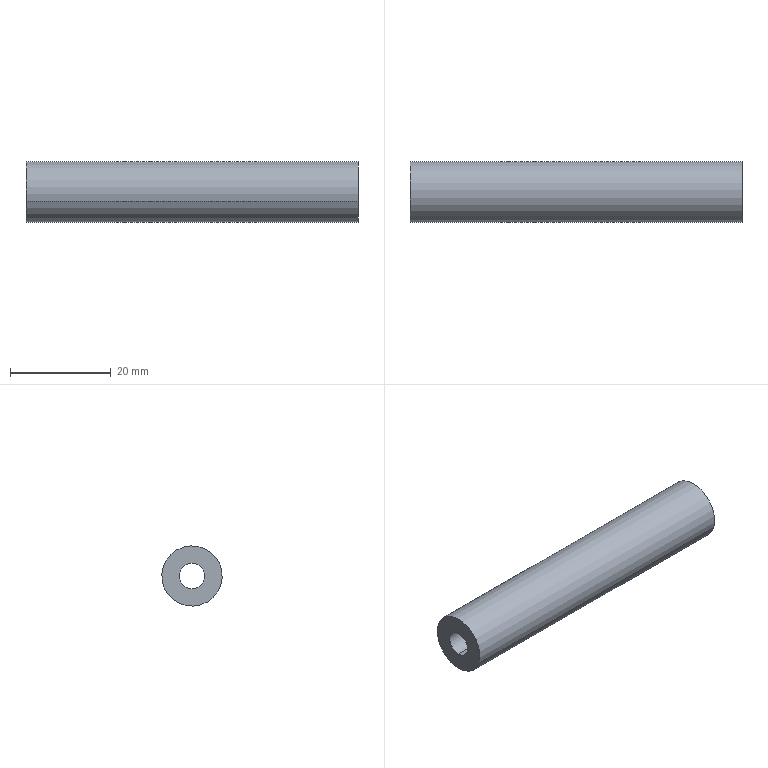Part | STEP file | Previa 01.sldasm-Part-10_Valor predeterminado | 1 solid | 6 faces | box 66 x 12 x 12 mm | volume 6169 mm3 | cylinder 4 | plane 2 | commonest cylinder face diameters 5 x2 12 x2
STEP:
#1=CARTESIAN_POINT('',(0.,0.,0.));
#2=DIRECTION('',(0.,0.,1.));
#3=DIRECTION('',(1.,0.,0.));
#4=AXIS2_PLACEMENT_3D('',#1,#2,#3);
#5=CARTESIAN_POINT('',(-100.103,41.846,11.097));
#6=VERTEX_POINT('',#5);
#7=CARTESIAN_POINT('',(-34.103,41.846,11.097));
#8=VERTEX_POINT('',#7);
#9=CARTESIAN_POINT('',(-34.103,41.846,11.097));
#10=DIRECTION('',(1.,0.,0.));
#11=VECTOR('',#10,1.);
#12=LINE('',#9,#11);
#13=CARTESIAN_POINT('',(-34.103,41.846,13.597));
#14=DIRECTION('',(1.,0.,0.));
#15=DIRECTION('',(0.,0.,-1.));
#16=AXIS2_PLACEMENT_3D('',#13,#14,#15);
#17=CYLINDRICAL_SURFACE('',#16,2.5);
#18=CARTESIAN_POINT('',(6.283,0.));
#19=DIRECTION('',(0.,1.));
#20=VECTOR('',#19,1.);
#21=LINE('',#18,#20);
#22=(GEOMETRIC_REPRESENTATION_CONTEXT(2)PARAMETRIC_REPRESENTATION_CONTEXT()REPRESENTATION_CONTEXT('',''));
#23=DEFINITIONAL_REPRESENTATION('',(#21),#22);
#24=PCURVE('',#17,#23);
#25=CARTESIAN_POINT('',(-34.103,41.846,13.597));
#26=DIRECTION('',(1.,0.,0.));
#27=DIRECTION('',(0.,0.,-1.));
#28=AXIS2_PLACEMENT_3D('',#25,#26,#27);
#29=CYLINDRICAL_SURFACE('',#28,2.5);
#30=CARTESIAN_POINT('',(0.,0.));
#31=DIRECTION('',(0.,1.));
#32=VECTOR('',#31,1.);
#33=LINE('',#30,#32);
#34=(GEOMETRIC_REPRESENTATION_CONTEXT(2)PARAMETRIC_REPRESENTATION_CONTEXT()REPRESENTATION_CONTEXT('',''));
#35=DEFINITIONAL_REPRESENTATION('',(#33),#34);
#36=PCURVE('',#29,#35);
#37=SURFACE_CURVE('',#12,(#24,#36),.PCURVE_S1.);
#38=EDGE_CURVE('',#6,#8,#37,.T.);
#39=ORIENTED_EDGE('',*,*,#38,.T.);
#40=CARTESIAN_POINT('',(-34.103,41.846,16.097));
#41=VERTEX_POINT('',#40);
#42=CARTESIAN_POINT('',(-34.103,41.846,13.597));
#43=DIRECTION('',(1.,0.,0.));
#44=DIRECTION('',(0.,0.,-1.));
#45=AXIS2_PLACEMENT_3D('',#42,#43,#44);
#46=CIRCLE('',#45,2.5);
#47=CARTESIAN_POINT('',(0.,0.));
#48=DIRECTION('',(1.,0.));
#49=VECTOR('',#48,1.);
#50=LINE('',#47,#49);
#51=(GEOMETRIC_REPRESENTATION_CONTEXT(2)PARAMETRIC_REPRESENTATION_CONTEXT()REPRESENTATION_CONTEXT('',''));
#52=DEFINITIONAL_REPRESENTATION('',(#50),#51);
#53=PCURVE('',#17,#52);
#54=CARTESIAN_POINT('',(-34.103,41.846,13.597));
#55=DIRECTION('',(-1.,0.,0.));
#56=DIRECTION('',(0.,0.9511,0.309));
#57=AXIS2_PLACEMENT_3D('',#54,#55,#56);
#58=PLANE('',#57);
#59=CARTESIAN_POINT('',(-0.7725,2.378));
#60=CARTESIAN_POINT('',(3.346,3.716));
#61=CARTESIAN_POINT('',(2.445,-0.5198));
#62=CARTESIAN_POINT('',(1.545,-4.755));
#63=CARTESIAN_POINT('',(-1.673,-1.858));
#64=CARTESIAN_POINT('',(-4.891,1.04));
#65=CARTESIAN_POINT('',(-0.7725,2.378));
#66=(BOUNDED_CURVE()B_SPLINE_CURVE(2,(#59,#60,#61,#62,#63,#64,#65),.UNSPECIFIED.,.T.,.F.)B_SPLINE_CURVE_WITH_KNOTS((1,2,2,2,2,1),(-2.094,0.,2.094,4.189,6.283,8.378),.UNSPECIFIED.)CURVE()GEOMETRIC_REPRESENTATION_ITEM()RATIONAL_B_SPLINE_CURVE((1.,0.5,1.,0.5,1.,0.5,1.))REPRESENTATION_ITEM(''));
#67=(GEOMETRIC_REPRESENTATION_CONTEXT(2)PARAMETRIC_REPRESENTATION_CONTEXT()REPRESENTATION_CONTEXT('',''));
#68=DEFINITIONAL_REPRESENTATION('',(#66),#67);
#69=PCURVE('',#58,#68);
#70=SURFACE_CURVE('',#46,(#53,#69),.PCURVE_S1.);
#71=EDGE_CURVE('',#41,#8,#70,.T.);
#72=ORIENTED_EDGE('',*,*,#71,.F.);
#73=CARTESIAN_POINT('',(-100.103,41.846,16.097));
#74=VERTEX_POINT('',#73);
#75=CARTESIAN_POINT('',(-34.103,41.846,16.097));
#76=DIRECTION('',(1.,0.,0.));
#77=VECTOR('',#76,1.);
#78=LINE('',#75,#77);
#79=CARTESIAN_POINT('',(3.142,0.));
#80=DIRECTION('',(0.,1.));
#81=VECTOR('',#80,1.);
#82=LINE('',#79,#81);
#83=(GEOMETRIC_REPRESENTATION_CONTEXT(2)PARAMETRIC_REPRESENTATION_CONTEXT()REPRESENTATION_CONTEXT('',''));
#84=DEFINITIONAL_REPRESENTATION('',(#82),#83);
#85=PCURVE('',#17,#84);
#86=CARTESIAN_POINT('',(3.142,0.));
#87=DIRECTION('',(0.,1.));
#88=VECTOR('',#87,1.);
#89=LINE('',#86,#88);
#90=(GEOMETRIC_REPRESENTATION_CONTEXT(2)PARAMETRIC_REPRESENTATION_CONTEXT()REPRESENTATION_CONTEXT('',''));
#91=DEFINITIONAL_REPRESENTATION('',(#89),#90);
#92=PCURVE('',#29,#91);
#93=SURFACE_CURVE('',#78,(#85,#92),.PCURVE_S1.);
#94=EDGE_CURVE('',#74,#41,#93,.T.);
#95=ORIENTED_EDGE('',*,*,#94,.F.);
#96=CARTESIAN_POINT('',(-100.103,41.846,13.597));
#97=DIRECTION('',(1.,0.,0.));
#98=DIRECTION('',(0.,0.,-1.));
#99=AXIS2_PLACEMENT_3D('',#96,#97,#98);
#100=CIRCLE('',#99,2.5);
#101=CARTESIAN_POINT('',(0.,-66.));
#102=DIRECTION('',(1.,0.));
#103=VECTOR('',#102,1.);
#104=LINE('',#101,#103);
#105=(GEOMETRIC_REPRESENTATION_CONTEXT(2)PARAMETRIC_REPRESENTATION_CONTEXT()REPRESENTATION_CONTEXT('',''));
#106=DEFINITIONAL_REPRESENTATION('',(#104),#105);
#107=PCURVE('',#17,#106);
#108=CARTESIAN_POINT('',(-100.103,41.846,13.597));
#109=DIRECTION('',(-1.,0.,0.));
#110=DIRECTION('',(0.,0.9511,0.309));
#111=AXIS2_PLACEMENT_3D('',#108,#109,#110);
#112=PLANE('',#111);
#113=CARTESIAN_POINT('',(-0.7725,2.378));
#114=CARTESIAN_POINT('',(3.346,3.716));
#115=CARTESIAN_POINT('',(2.445,-0.5198));
#116=CARTESIAN_POINT('',(1.545,-4.755));
#117=CARTESIAN_POINT('',(-1.673,-1.858));
#118=CARTESIAN_POINT('',(-4.891,1.04));
#119=CARTESIAN_POINT('',(-0.7725,2.378));
#120=(BOUNDED_CURVE()B_SPLINE_CURVE(2,(#113,#114,#115,#116,#117,#118,#119),.UNSPECIFIED.,.T.,.F.)B_SPLINE_CURVE_WITH_KNOTS((1,2,2,2,2,1),(-2.094,0.,2.094,4.189,6.283,8.378),.UNSPECIFIED.)CURVE()GEOMETRIC_REPRESENTATION_ITEM()RATIONAL_B_SPLINE_CURVE((1.,0.5,1.,0.5,1.,0.5,1.))REPRESENTATION_ITEM(''));
#121=(GEOMETRIC_REPRESENTATION_CONTEXT(2)PARAMETRIC_REPRESENTATION_CONTEXT()REPRESENTATION_CONTEXT('',''));
#122=DEFINITIONAL_REPRESENTATION('',(#120),#121);
#123=PCURVE('',#112,#122);
#124=SURFACE_CURVE('',#100,(#107,#123),.PCURVE_S1.);
#125=EDGE_CURVE('',#74,#6,#124,.T.);
#126=ORIENTED_EDGE('',*,*,#125,.T.);
#127=EDGE_LOOP('',(#39,#72,#95,#126));
#128=FACE_BOUND('',#127,.F.);
#129=ADVANCED_FACE('',(#128),#17,.F.);
#130=CARTESIAN_POINT('',(-100.103,47.553,15.451));
#131=VERTEX_POINT('',#130);
#132=CARTESIAN_POINT('',(-100.103,36.14,11.743));
#133=VERTEX_POINT('',#132);
#134=CARTESIAN_POINT('',(-100.103,41.846,13.597));
#135=DIRECTION('',(-1.,0.,0.));
#136=DIRECTION('',(0.,0.,1.));
#137=AXIS2_PLACEMENT_3D('',#134,#135,#136);
#138=CIRCLE('',#137,6.);
#139=CARTESIAN_POINT('',(-162.103,41.846,13.597));
#140=DIRECTION('',(1.,0.,0.));
#141=DIRECTION('',(0.,-0.9511,-0.309));
#142=AXIS2_PLACEMENT_3D('',#139,#140,#141);
#143=CYLINDRICAL_SURFACE('',#142,6.);
#144=CARTESIAN_POINT('',(4.398,62.));
#145=DIRECTION('',(-1.,0.));
#146=VECTOR('',#145,1.);
#147=LINE('',#144,#146);
#148=(GEOMETRIC_REPRESENTATION_CONTEXT(2)PARAMETRIC_REPRESENTATION_CONTEXT()REPRESENTATION_CONTEXT('',''));
#149=DEFINITIONAL_REPRESENTATION('',(#147),#148);
#150=PCURVE('',#143,#149);
#151=CARTESIAN_POINT('',(0.,0.));
#152=DIRECTION('',(0.309,-0.9511));
#153=AXIS2_PLACEMENT_2D('',#151,#152);
#154=CIRCLE('',#153,6.);
#155=(GEOMETRIC_REPRESENTATION_CONTEXT(2)PARAMETRIC_REPRESENTATION_CONTEXT()REPRESENTATION_CONTEXT('',''));
#156=DEFINITIONAL_REPRESENTATION('',(#154),#155);
#157=PCURVE('',#112,#156);
#158=SURFACE_CURVE('',#138,(#150,#157),.PCURVE_S1.);
#159=EDGE_CURVE('',#131,#133,#158,.T.);
#160=ORIENTED_EDGE('',*,*,#159,.F.);
#161=CARTESIAN_POINT('',(-34.103,47.553,15.451));
#162=VERTEX_POINT('',#161);
#163=CARTESIAN_POINT('',(-162.103,47.553,15.451));
#164=DIRECTION('',(1.,0.,0.));
#165=VECTOR('',#164,1.);
#166=LINE('',#163,#165);
#167=CARTESIAN_POINT('',(3.142,0.));
#168=DIRECTION('',(0.,1.));
#169=VECTOR('',#168,1.);
#170=LINE('',#167,#169);
#171=(GEOMETRIC_REPRESENTATION_CONTEXT(2)PARAMETRIC_REPRESENTATION_CONTEXT()REPRESENTATION_CONTEXT('',''));
#172=DEFINITIONAL_REPRESENTATION('',(#170),#171);
#173=PCURVE('',#143,#172);
#174=CARTESIAN_POINT('',(-162.103,41.846,13.597));
#175=DIRECTION('',(1.,0.,0.));
#176=DIRECTION('',(0.,-0.9511,-0.309));
#177=AXIS2_PLACEMENT_3D('',#174,#175,#176);
#178=CYLINDRICAL_SURFACE('',#177,6.);
#179=CARTESIAN_POINT('',(3.142,0.));
#180=DIRECTION('',(0.,1.));
#181=VECTOR('',#180,1.);
#182=LINE('',#179,#181);
#183=(GEOMETRIC_REPRESENTATION_CONTEXT(2)PARAMETRIC_REPRESENTATION_CONTEXT()REPRESENTATION_CONTEXT('',''));
#184=DEFINITIONAL_REPRESENTATION('',(#182),#183);
#185=PCURVE('',#178,#184);
#186=SURFACE_CURVE('',#166,(#173,#185),.PCURVE_S1.);
#187=EDGE_CURVE('',#131,#162,#186,.T.);
#188=ORIENTED_EDGE('',*,*,#187,.T.);
#189=CARTESIAN_POINT('',(-34.103,36.14,11.743));
#190=VERTEX_POINT('',#189);
#191=CARTESIAN_POINT('',(-34.103,41.846,13.597));
#192=DIRECTION('',(-1.,0.,0.));
#193=DIRECTION('',(0.,-0.309,0.9511));
#194=AXIS2_PLACEMENT_3D('',#191,#192,#193);
#195=CIRCLE('',#194,6.);
#196=CARTESIAN_POINT('',(4.712,128.));
#197=DIRECTION('',(-1.,0.));
#198=VECTOR('',#197,1.);
#199=LINE('',#196,#198);
#200=(GEOMETRIC_REPRESENTATION_CONTEXT(2)PARAMETRIC_REPRESENTATION_CONTEXT()REPRESENTATION_CONTEXT('',''));
#201=DEFINITIONAL_REPRESENTATION('',(#199),#200);
#202=PCURVE('',#143,#201);
#203=CARTESIAN_POINT('',(0.,0.));
#204=DIRECTION('',(0.,-1.));
#205=AXIS2_PLACEMENT_2D('',#203,#204);
#206=CIRCLE('',#205,6.);
#207=(GEOMETRIC_REPRESENTATION_CONTEXT(2)PARAMETRIC_REPRESENTATION_CONTEXT()REPRESENTATION_CONTEXT('',''));
#208=DEFINITIONAL_REPRESENTATION('',(#206),#207);
#209=PCURVE('',#58,#208);
#210=SURFACE_CURVE('',#195,(#202,#209),.PCURVE_S1.);
#211=EDGE_CURVE('',#162,#190,#210,.T.);
#212=ORIENTED_EDGE('',*,*,#211,.T.);
#213=CARTESIAN_POINT('',(-162.103,36.14,11.743));
#214=DIRECTION('',(1.,0.,0.));
#215=VECTOR('',#214,1.);
#216=LINE('',#213,#215);
#217=CARTESIAN_POINT('',(0.,0.));
#218=DIRECTION('',(0.,1.));
#219=VECTOR('',#218,1.);
#220=LINE('',#217,#219);
#221=(GEOMETRIC_REPRESENTATION_CONTEXT(2)PARAMETRIC_REPRESENTATION_CONTEXT()REPRESENTATION_CONTEXT('',''));
#222=DEFINITIONAL_REPRESENTATION('',(#220),#221);
#223=PCURVE('',#143,#222);
#224=CARTESIAN_POINT('',(6.283,0.));
#225=DIRECTION('',(0.,1.));
#226=VECTOR('',#225,1.);
#227=LINE('',#224,#226);
#228=(GEOMETRIC_REPRESENTATION_CONTEXT(2)PARAMETRIC_REPRESENTATION_CONTEXT()REPRESENTATION_CONTEXT('',''));
#229=DEFINITIONAL_REPRESENTATION('',(#227),#228);
#230=PCURVE('',#178,#229);
#231=SURFACE_CURVE('',#216,(#223,#230),.PCURVE_S1.);
#232=EDGE_CURVE('',#133,#190,#231,.T.);
#233=ORIENTED_EDGE('',*,*,#232,.F.);
#234=EDGE_LOOP('',(#160,#188,#212,#233));
#235=FACE_BOUND('',#234,.T.);
#236=ADVANCED_FACE('',(#235),#143,.T.);
#237=ORIENTED_EDGE('',*,*,#187,.F.);
#238=CARTESIAN_POINT('',(-100.103,41.846,13.597));
#239=DIRECTION('',(-1.,0.,0.));
#240=DIRECTION('',(0.,0.,1.));
#241=AXIS2_PLACEMENT_3D('',#238,#239,#240);
#242=CIRCLE('',#241,6.);
#243=CARTESIAN_POINT('',(10.681,62.));
#244=DIRECTION('',(-1.,0.));
#245=VECTOR('',#244,1.);
#246=LINE('',#243,#245);
#247=(GEOMETRIC_REPRESENTATION_CONTEXT(2)PARAMETRIC_REPRESENTATION_CONTEXT()REPRESENTATION_CONTEXT('',''));
#248=DEFINITIONAL_REPRESENTATION('',(#246),#247);
#249=PCURVE('',#178,#248);
#250=CARTESIAN_POINT('',(0.,0.));
#251=DIRECTION('',(0.309,-0.9511));
#252=AXIS2_PLACEMENT_2D('',#250,#251);
#253=CIRCLE('',#252,6.);
#254=(GEOMETRIC_REPRESENTATION_CONTEXT(2)PARAMETRIC_REPRESENTATION_CONTEXT()REPRESENTATION_CONTEXT('',''));
#255=DEFINITIONAL_REPRESENTATION('',(#253),#254);
#256=PCURVE('',#112,#255);
#257=SURFACE_CURVE('',#242,(#249,#256),.PCURVE_S1.);
#258=EDGE_CURVE('',#133,#131,#257,.T.);
#259=ORIENTED_EDGE('',*,*,#258,.F.);
#260=ORIENTED_EDGE('',*,*,#232,.T.);
#261=CARTESIAN_POINT('',(-34.103,41.846,13.597));
#262=DIRECTION('',(-1.,0.,0.));
#263=DIRECTION('',(0.,-0.309,0.9511));
#264=AXIS2_PLACEMENT_3D('',#261,#262,#263);
#265=CIRCLE('',#264,6.);
#266=CARTESIAN_POINT('',(10.996,128.));
#267=DIRECTION('',(-1.,0.));
#268=VECTOR('',#267,1.);
#269=LINE('',#266,#268);
#270=(GEOMETRIC_REPRESENTATION_CONTEXT(2)PARAMETRIC_REPRESENTATION_CONTEXT()REPRESENTATION_CONTEXT('',''));
#271=DEFINITIONAL_REPRESENTATION('',(#269),#270);
#272=PCURVE('',#178,#271);
#273=CARTESIAN_POINT('',(0.,0.));
#274=DIRECTION('',(0.,-1.));
#275=AXIS2_PLACEMENT_2D('',#273,#274);
#276=CIRCLE('',#275,6.);
#277=(GEOMETRIC_REPRESENTATION_CONTEXT(2)PARAMETRIC_REPRESENTATION_CONTEXT()REPRESENTATION_CONTEXT('',''));
#278=DEFINITIONAL_REPRESENTATION('',(#276),#277);
#279=PCURVE('',#58,#278);
#280=SURFACE_CURVE('',#265,(#272,#279),.PCURVE_S1.);
#281=EDGE_CURVE('',#190,#162,#280,.T.);
#282=ORIENTED_EDGE('',*,*,#281,.T.);
#283=EDGE_LOOP('',(#237,#259,#260,#282));
#284=FACE_BOUND('',#283,.T.);
#285=ADVANCED_FACE('',(#284),#178,.T.);
#286=CARTESIAN_POINT('',(-100.103,41.846,13.597));
#287=DIRECTION('',(1.,0.,0.));
#288=DIRECTION('',(0.,0.,-1.));
#289=AXIS2_PLACEMENT_3D('',#286,#287,#288);
#290=CIRCLE('',#289,2.5);
#291=CARTESIAN_POINT('',(-0.7725,2.378));
#292=CARTESIAN_POINT('',(3.346,3.716));
#293=CARTESIAN_POINT('',(2.445,-0.5198));
#294=CARTESIAN_POINT('',(1.545,-4.755));
#295=CARTESIAN_POINT('',(-1.673,-1.858));
#296=CARTESIAN_POINT('',(-4.891,1.04));
#297=CARTESIAN_POINT('',(-0.7725,2.378));
#298=(BOUNDED_CURVE()B_SPLINE_CURVE(2,(#291,#292,#293,#294,#295,#296,#297),.UNSPECIFIED.,.T.,.F.)B_SPLINE_CURVE_WITH_KNOTS((1,2,2,2,2,1),(-2.094,0.,2.094,4.189,6.283,8.378),.UNSPECIFIED.)CURVE()GEOMETRIC_REPRESENTATION_ITEM()RATIONAL_B_SPLINE_CURVE((1.,0.5,1.,0.5,1.,0.5,1.))REPRESENTATION_ITEM(''));
#299=(GEOMETRIC_REPRESENTATION_CONTEXT(2)PARAMETRIC_REPRESENTATION_CONTEXT()REPRESENTATION_CONTEXT('',''));
#300=DEFINITIONAL_REPRESENTATION('',(#298),#299);
#301=PCURVE('',#112,#300);
#302=CARTESIAN_POINT('',(0.,-66.));
#303=DIRECTION('',(1.,0.));
#304=VECTOR('',#303,1.);
#305=LINE('',#302,#304);
#306=(GEOMETRIC_REPRESENTATION_CONTEXT(2)PARAMETRIC_REPRESENTATION_CONTEXT()REPRESENTATION_CONTEXT('',''));
#307=DEFINITIONAL_REPRESENTATION('',(#305),#306);
#308=PCURVE('',#29,#307);
#309=SURFACE_CURVE('',#290,(#301,#308),.PCURVE_S1.);
#310=EDGE_CURVE('',#6,#74,#309,.T.);
#311=ORIENTED_EDGE('',*,*,#310,.T.);
#312=ORIENTED_EDGE('',*,*,#125,.T.);
#313=EDGE_LOOP('',(#311,#312));
#314=FACE_BOUND('',#313,.T.);
#315=ORIENTED_EDGE('',*,*,#258,.T.);
#316=ORIENTED_EDGE('',*,*,#159,.T.);
#317=EDGE_LOOP('',(#315,#316));
#318=FACE_BOUND('',#317,.T.);
#319=ADVANCED_FACE('',(#314,#318),#112,.T.);
#320=CARTESIAN_POINT('',(-34.103,41.846,13.597));
#321=DIRECTION('',(1.,0.,0.));
#322=DIRECTION('',(0.,0.,-1.));
#323=AXIS2_PLACEMENT_3D('',#320,#321,#322);
#324=CIRCLE('',#323,2.5);
#325=CARTESIAN_POINT('',(-0.7725,2.378));
#326=CARTESIAN_POINT('',(3.346,3.716));
#327=CARTESIAN_POINT('',(2.445,-0.5198));
#328=CARTESIAN_POINT('',(1.545,-4.755));
#329=CARTESIAN_POINT('',(-1.673,-1.858));
#330=CARTESIAN_POINT('',(-4.891,1.04));
#331=CARTESIAN_POINT('',(-0.7725,2.378));
#332=(BOUNDED_CURVE()B_SPLINE_CURVE(2,(#325,#326,#327,#328,#329,#330,#331),.UNSPECIFIED.,.T.,.F.)B_SPLINE_CURVE_WITH_KNOTS((1,2,2,2,2,1),(-2.094,0.,2.094,4.189,6.283,8.378),.UNSPECIFIED.)CURVE()GEOMETRIC_REPRESENTATION_ITEM()RATIONAL_B_SPLINE_CURVE((1.,0.5,1.,0.5,1.,0.5,1.))REPRESENTATION_ITEM(''));
#333=(GEOMETRIC_REPRESENTATION_CONTEXT(2)PARAMETRIC_REPRESENTATION_CONTEXT()REPRESENTATION_CONTEXT('',''));
#334=DEFINITIONAL_REPRESENTATION('',(#332),#333);
#335=PCURVE('',#58,#334);
#336=CARTESIAN_POINT('',(0.,0.));
#337=DIRECTION('',(1.,0.));
#338=VECTOR('',#337,1.);
#339=LINE('',#336,#338);
#340=(GEOMETRIC_REPRESENTATION_CONTEXT(2)PARAMETRIC_REPRESENTATION_CONTEXT()REPRESENTATION_CONTEXT('',''));
#341=DEFINITIONAL_REPRESENTATION('',(#339),#340);
#342=PCURVE('',#29,#341);
#343=SURFACE_CURVE('',#324,(#335,#342),.PCURVE_S1.);
#344=EDGE_CURVE('',#8,#41,#343,.T.);
#345=ORIENTED_EDGE('',*,*,#344,.F.);
#346=ORIENTED_EDGE('',*,*,#71,.F.);
#347=EDGE_LOOP('',(#345,#346));
#348=FACE_BOUND('',#347,.T.);
#349=ORIENTED_EDGE('',*,*,#281,.F.);
#350=ORIENTED_EDGE('',*,*,#211,.F.);
#351=EDGE_LOOP('',(#349,#350));
#352=FACE_BOUND('',#351,.T.);
#353=ADVANCED_FACE('',(#348,#352),#58,.F.);
#354=ORIENTED_EDGE('',*,*,#344,.F.);
#355=ORIENTED_EDGE('',*,*,#38,.F.);
#356=ORIENTED_EDGE('',*,*,#310,.T.);
#357=ORIENTED_EDGE('',*,*,#94,.T.);
#358=EDGE_LOOP('',(#354,#355,#356,#357));
#359=FACE_BOUND('',#358,.F.);
#360=ADVANCED_FACE('',(#359),#29,.F.);
#361=CLOSED_SHELL('',(#129,#236,#285,#319,#353,#360));
#362=MANIFOLD_SOLID_BREP('',#361);
#363=(LENGTH_UNIT()NAMED_UNIT(*)SI_UNIT(.MILLI.,.METRE.));
#364=UNCERTAINTY_MEASURE_WITH_UNIT(LENGTH_MEASURE(0.0000001),#363,'','');
#365=(NAMED_UNIT(*)PLANE_ANGLE_UNIT()SI_UNIT($,.RADIAN.));
#366=(NAMED_UNIT(*)SI_UNIT($,.STERADIAN.)SOLID_ANGLE_UNIT());
#367=(GEOMETRIC_REPRESENTATION_CONTEXT(3)GLOBAL_UNCERTAINTY_ASSIGNED_CONTEXT((#364))GLOBAL_UNIT_ASSIGNED_CONTEXT((#363,#365,#366))REPRESENTATION_CONTEXT('',''));
#368=ADVANCED_BREP_SHAPE_REPRESENTATION('',(#4,#362),#367);